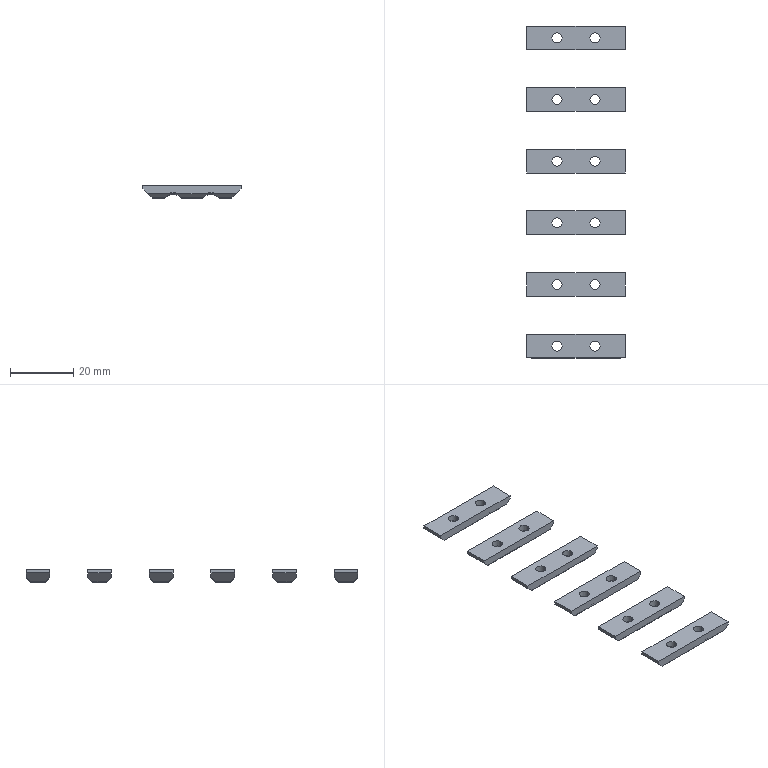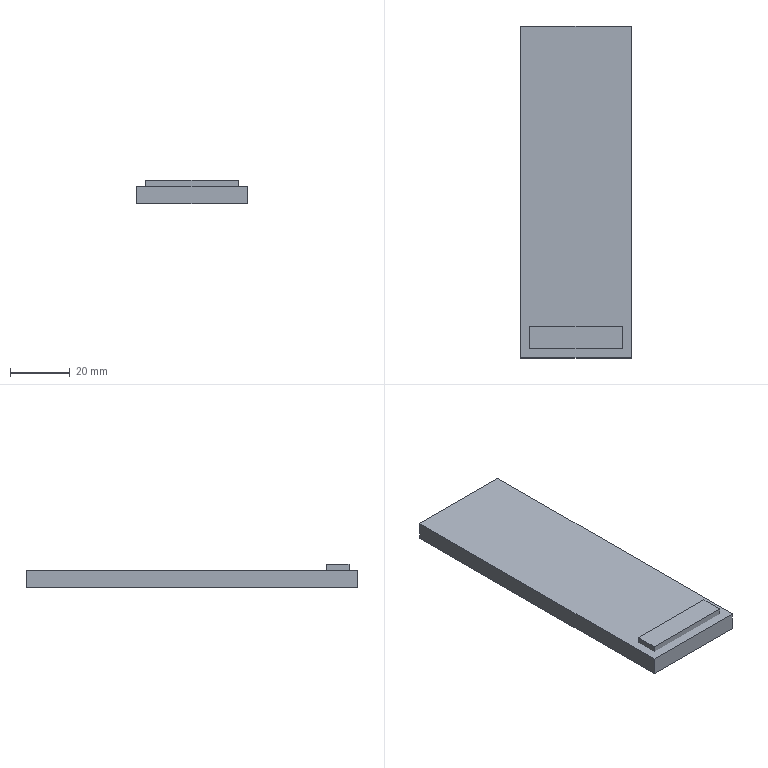CAM job | NX | 3-axis milling, drilling | part box 31 x 105 x 4 mm | stock box 37 x 111 x 8 mm
Tools:
number,name,description,diameter,corner_radius,flute_length,length,flutes
15,D10,Milling Tool-5 Parameters,10.0,0.0,50.0,75.0,2
14,D10JING,Milling Tool-5 Parameters,10.0,0.0,50.0,75.0,2
1,D6A45,Milling Tool-5 Parameters,6.0,0.0,50.0,75.0,2
3,3.2ZT,Drilling Tool,3.2,0.0,35.0,50.0,2
11,D4,Milling Tool-5 Parameters,4.0,0.0,50.0,75.0,2
16,D4R0.5,Milling Tool-5 Parameters,4.0,0.5,50.0,75.0,2
17,D0.3,Milling Tool-5 Parameters,0.3,0.0,50.0,75.0,2
Operations:
program,operation,operation_type,tool,method,geometry_group,spindle_rpm,surface_speed,feed_per_tooth,feed_cut,feed_plunge,cut_length_mm,path_length_mm,cut_time_min,machine_time_min
1,FLOOR_WALL_COPY,VolumeBased25DMillingOperation,D10JING,METHOD,A,9500.0,298.0,0.0789,1500.0,100.0,1549.994,1688.991,1.033,1.047
1,ZLEVEL_PROFILE_1,ZLevelMilling,D10,METHOD,A,9500.0,298.0,0.1316,2500.0,1000.0,3187.718,3729.789,1.437,1.491
1,DRILLING_COPY_1,Operation,D6A45,METHOD,A,5000.0,94.0,0.035,350.0,0.0,48.0,361.863,0.1371,0.1685
1,DRILLING_COPY_COPY_COPY_2,Operation,3.2ZT,METHOD,A,2000.0,20.0,0.045,180.0,0.0,113.537,492.936,0.6308,0.6687
1,HOLE_MILLING,CylinderMilling,D4,METHOD,A,9500.0,119.0,0.0658,1250.0,100.0,1018.64,1920.14,0.8149,0.9051
1,ZLEVEL_PROFILE,ZLevelMilling,D4R0.5,METHOD,A,9500.0,119.0,0.1316,2500.0,100.0,4654.305,5591.338,1.862,1.955
1,ZLEVEL_PROFILE_COPY,ZLevelMilling,D4R0.5,METHOD,A,9500.0,119.0,0.1316,2500.0,100.0,11234.937,12129.134,4.494,4.583
1,PLANAR_MILL,PlanarMilling,D0.3,METHOD,A,9500.0,8.0,0.0395,750.0,100.0,1279.0,10722.217,1.705,2.65
1,PLANAR_MILL_COPY,PlanarMilling,D0.3,METHOD,A,9500.0,8.0,0.0395,750.0,100.0,1279.0,10722.217,1.705,2.65
1,PLANAR_MILL_COPY_1,PlanarMilling,D0.3,METHOD,A,9500.0,8.0,0.0395,750.0,100.0,1279.0,10722.217,1.705,2.65
1,PLANAR_MILL_COPY_2,PlanarMilling,D0.3,METHOD,A,9500.0,8.0,0.0395,750.0,100.0,1279.0,10722.217,1.705,2.65
1,PLANAR_MILL_COPY_3,PlanarMilling,D0.3,METHOD,A,9500.0,8.0,0.0395,750.0,100.0,1279.0,10722.217,1.705,2.65
1,PLANAR_MILL_COPY_4,PlanarMilling,D0.3,METHOD,A,9500.0,8.0,0.0395,750.0,100.0,1279.0,10722.217,1.705,2.65
1,ZLEVEL_PROFILE_1_COPY,ZLevelMilling,D10JING,METHOD,A,9500.0,298.0,0.0632,1200.0,1000.0,2840.266,3498.885,2.398,2.464
2,FLOOR_WALL_COPY_COPY,VolumeBased25DMillingOperation,D10JING,METHOD,B,51980.0,1633.0,0.0144,1500.0,100.0,405.988,620.48,0.2707,0.2921
2,PLANAR_MILL_COPY_COPY_COPY_COPY_COPY_COPY_1_COPY,PlanarMilling,D6A45,METHOD,B,9500.0,179.0,0.0658,1250.0,100.0,104.64,300.04,0.0837,0.1033